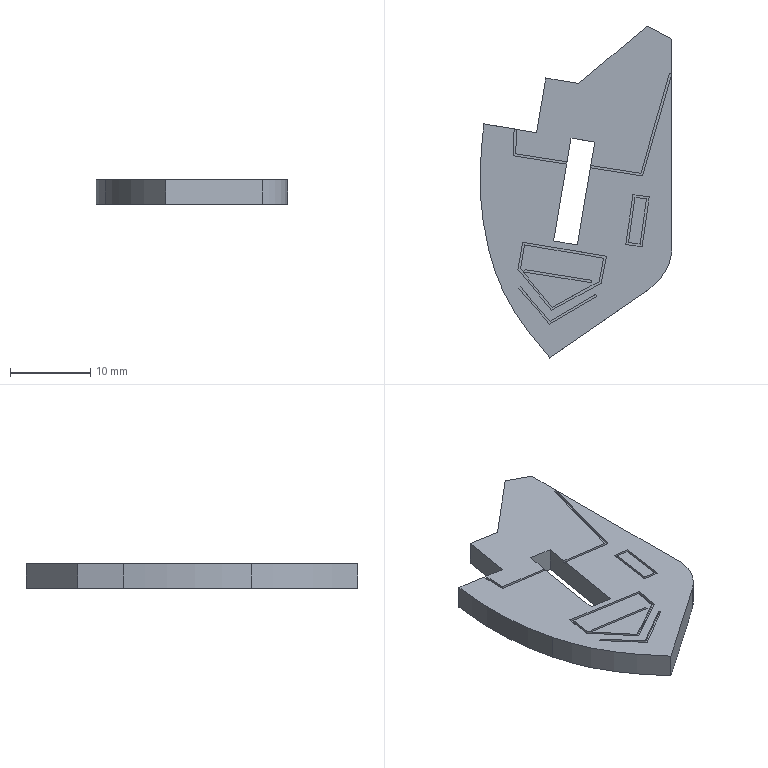Part | SolidWorks | features BaseBody 1 | 1 solid | 63 faces | box 23.87 x 41.361 x 3 mm | volume 1927 mm3 | plane 58 | spline 5